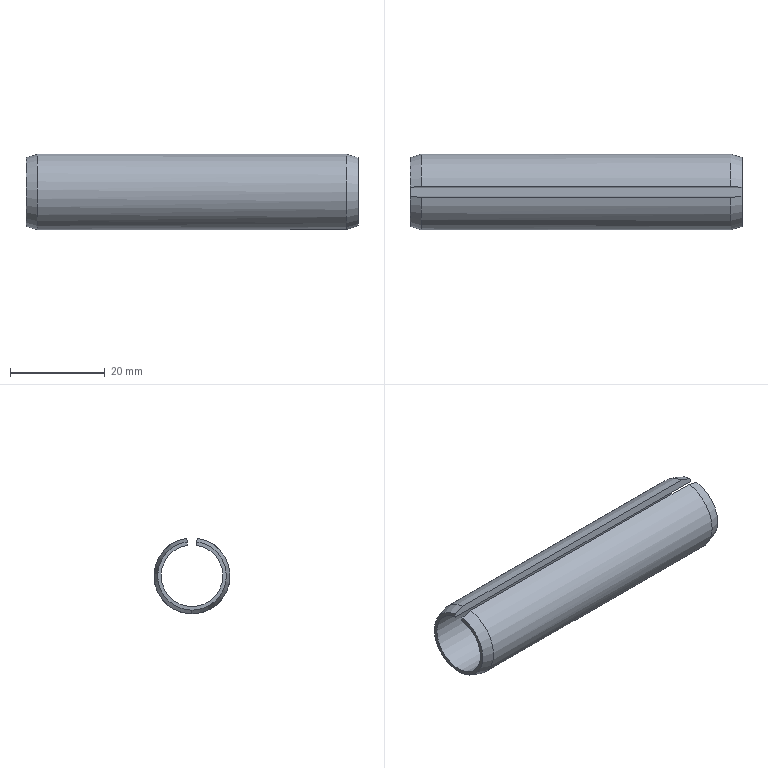Part | SolidWorks | features Boss 1, Cut 1, Extrusion 1, RevCut 1 | 1 solid | 9 faces | box 70 x 16 x 15.922 mm | volume 4487 mm3 | plane 4 | cone 3 | cylinder 2 | commonest cylinder face diameters 13 x1 16 x1
STEP:
#1=CARTESIAN_POINT('',(0.,-1.009,7.179));
#2=VERTEX_POINT('',#1);
#3=CARTESIAN_POINT('',(0.,0.,-7.25));
#4=VERTEX_POINT('',#3);
#5=CARTESIAN_POINT('',(0.,0.,0.));
#6=DIRECTION('',(1.,0.,0.));
#7=DIRECTION('',(0.,0.,-1.));
#8=AXIS2_PLACEMENT_3D('',#5,#6,#7);
#9=CIRCLE('',#8,7.25);
#10=EDGE_CURVE('',#2,#4,#9,.T.);
#11=ORIENTED_EDGE('',*,*,#10,.T.);
#12=CARTESIAN_POINT('',(2.4,0.,-8.));
#13=VERTEX_POINT('',#12);
#14=CARTESIAN_POINT('',(0.,0.,-7.25));
#15=DIRECTION('',(0.9545,0.,-0.2983));
#16=VECTOR('',#15,1000.);
#17=LINE('',#14,#16);
#18=EDGE_CURVE('',#4,#13,#17,.T.);
#19=ORIENTED_EDGE('',*,*,#18,.T.);
#20=CARTESIAN_POINT('',(2.4,-1.113,7.922));
#21=VERTEX_POINT('',#20);
#22=CARTESIAN_POINT('',(2.4,0.,0.));
#23=DIRECTION('',(1.,0.,0.));
#24=DIRECTION('',(0.,0.,-1.));
#25=AXIS2_PLACEMENT_3D('',#22,#23,#24);
#26=CIRCLE('',#25,8.);
#27=EDGE_CURVE('',#21,#13,#26,.T.);
#28=ORIENTED_EDGE('',*,*,#27,.F.);
#29=CARTESIAN_POINT('',(-23.2,0.,0.));
#30=DIRECTION('',(0.9545,-0.04151,0.2954));
#31=VECTOR('',#30,1000.);
#32=LINE('',#29,#31);
#33=EDGE_CURVE('',#2,#21,#32,.T.);
#34=ORIENTED_EDGE('',*,*,#33,.F.);
#35=EDGE_LOOP('',(#11,#19,#28,#34));
#36=FACE_OUTER_BOUND('',#35,.T.);
#37=CARTESIAN_POINT('',(0.,0.,0.));
#38=DIRECTION('',(1.,0.,0.));
#39=DIRECTION('',(0.,0.,-1.));
#40=AXIS2_PLACEMENT_3D('',#37,#38,#39);
#41=CONICAL_SURFACE('',#40,7.25,0.3029);
#42=ADVANCED_FACE('',(#36),#41,.T.);
#43=CARTESIAN_POINT('',(70.,-0.9046,6.437));
#44=VERTEX_POINT('',#43);
#45=CARTESIAN_POINT('',(70.,0.9046,6.437));
#46=VERTEX_POINT('',#45);
#47=CARTESIAN_POINT('',(70.,0.,0.));
#48=DIRECTION('',(1.,0.,0.));
#49=DIRECTION('',(0.,0.,-1.));
#50=AXIS2_PLACEMENT_3D('',#47,#48,#49);
#51=CIRCLE('',#50,6.5);
#52=EDGE_CURVE('',#44,#46,#51,.T.);
#53=ORIENTED_EDGE('',*,*,#52,.F.);
#54=CARTESIAN_POINT('',(70.,-1.009,7.179));
#55=VERTEX_POINT('',#54);
#56=CARTESIAN_POINT('',(70.,0.,0.));
#57=DIRECTION('',(0.,0.1392,-0.9903));
#58=VECTOR('',#57,1000.);
#59=LINE('',#56,#58);
#60=EDGE_CURVE('',#55,#44,#59,.T.);
#61=ORIENTED_EDGE('',*,*,#60,.F.);
#62=CARTESIAN_POINT('',(70.,1.009,7.179));
#63=VERTEX_POINT('',#62);
#64=CARTESIAN_POINT('',(70.,0.,0.));
#65=DIRECTION('',(1.,0.,0.));
#66=DIRECTION('',(0.,0.,-1.));
#67=AXIS2_PLACEMENT_3D('',#64,#65,#66);
#68=CIRCLE('',#67,7.25);
#69=EDGE_CURVE('',#55,#63,#68,.T.);
#70=ORIENTED_EDGE('',*,*,#69,.T.);
#71=CARTESIAN_POINT('',(70.,0.,0.));
#72=DIRECTION('',(0.,0.1392,0.9903));
#73=VECTOR('',#72,1000.);
#74=LINE('',#71,#73);
#75=EDGE_CURVE('',#46,#63,#74,.T.);
#76=ORIENTED_EDGE('',*,*,#75,.F.);
#77=EDGE_LOOP('',(#53,#61,#70,#76));
#78=FACE_OUTER_BOUND('',#77,.T.);
#79=CARTESIAN_POINT('',(70.,0.,0.));
#80=DIRECTION('',(1.,0.,0.));
#81=DIRECTION('',(0.,0.,-1.));
#82=AXIS2_PLACEMENT_3D('',#79,#80,#81);
#83=PLANE('',#82);
#84=ADVANCED_FACE('',(#78),#83,.T.);
#85=CARTESIAN_POINT('',(0.,-0.9046,6.437));
#86=VERTEX_POINT('',#85);
#87=CARTESIAN_POINT('',(0.,0.,0.));
#88=DIRECTION('',(0.,0.1392,-0.9903));
#89=VECTOR('',#88,1000.);
#90=LINE('',#87,#89);
#91=EDGE_CURVE('',#2,#86,#90,.T.);
#92=ORIENTED_EDGE('',*,*,#91,.T.);
#93=CARTESIAN_POINT('',(0.,0.9046,6.437));
#94=VERTEX_POINT('',#93);
#95=CARTESIAN_POINT('',(0.,0.,0.));
#96=DIRECTION('',(1.,0.,0.));
#97=DIRECTION('',(0.,0.,-1.));
#98=AXIS2_PLACEMENT_3D('',#95,#96,#97);
#99=CIRCLE('',#98,6.5);
#100=EDGE_CURVE('',#86,#94,#99,.T.);
#101=ORIENTED_EDGE('',*,*,#100,.T.);
#102=CARTESIAN_POINT('',(0.,1.009,7.179));
#103=VERTEX_POINT('',#102);
#104=CARTESIAN_POINT('',(0.,0.,0.));
#105=DIRECTION('',(0.,0.1392,0.9903));
#106=VECTOR('',#105,1000.);
#107=LINE('',#104,#106);
#108=EDGE_CURVE('',#94,#103,#107,.T.);
#109=ORIENTED_EDGE('',*,*,#108,.T.);
#110=CARTESIAN_POINT('',(0.,0.,0.));
#111=DIRECTION('',(1.,0.,0.));
#112=DIRECTION('',(0.,0.,-1.));
#113=AXIS2_PLACEMENT_3D('',#110,#111,#112);
#114=CIRCLE('',#113,7.25);
#115=EDGE_CURVE('',#4,#103,#114,.T.);
#116=ORIENTED_EDGE('',*,*,#115,.F.);
#117=ORIENTED_EDGE('',*,*,#10,.F.);
#118=EDGE_LOOP('',(#92,#101,#109,#116,#117));
#119=FACE_OUTER_BOUND('',#118,.T.);
#120=CARTESIAN_POINT('',(0.,0.,0.));
#121=DIRECTION('',(1.,0.,0.));
#122=DIRECTION('',(0.,0.,-1.));
#123=AXIS2_PLACEMENT_3D('',#120,#121,#122);
#124=PLANE('',#123);
#125=ADVANCED_FACE('',(#119),#124,.F.);
#126=CARTESIAN_POINT('',(67.6,-1.113,7.922));
#127=VERTEX_POINT('',#126);
#128=CARTESIAN_POINT('',(70.,-1.113,7.922));
#129=DIRECTION('',(1.,0.,0.));
#130=VECTOR('',#129,1000.);
#131=LINE('',#128,#130);
#132=EDGE_CURVE('',#21,#127,#131,.T.);
#133=ORIENTED_EDGE('',*,*,#132,.F.);
#134=ORIENTED_EDGE('',*,*,#27,.T.);
#135=CARTESIAN_POINT('',(2.4,1.113,7.922));
#136=VERTEX_POINT('',#135);
#137=CARTESIAN_POINT('',(2.4,0.,0.));
#138=DIRECTION('',(1.,0.,0.));
#139=DIRECTION('',(0.,0.,-1.));
#140=AXIS2_PLACEMENT_3D('',#137,#138,#139);
#141=CIRCLE('',#140,8.);
#142=EDGE_CURVE('',#13,#136,#141,.T.);
#143=ORIENTED_EDGE('',*,*,#142,.T.);
#144=CARTESIAN_POINT('',(67.6,1.113,7.922));
#145=VERTEX_POINT('',#144);
#146=CARTESIAN_POINT('',(70.,1.113,7.922));
#147=DIRECTION('',(-1.,0.,0.));
#148=VECTOR('',#147,1000.);
#149=LINE('',#146,#148);
#150=EDGE_CURVE('',#145,#136,#149,.T.);
#151=ORIENTED_EDGE('',*,*,#150,.F.);
#152=CARTESIAN_POINT('',(67.6,0.,0.));
#153=DIRECTION('',(1.,0.,0.));
#154=DIRECTION('',(0.,0.,-1.));
#155=AXIS2_PLACEMENT_3D('',#152,#153,#154);
#156=CIRCLE('',#155,8.);
#157=EDGE_CURVE('',#127,#145,#156,.T.);
#158=ORIENTED_EDGE('',*,*,#157,.F.);
#159=EDGE_LOOP('',(#133,#134,#143,#151,#158));
#160=FACE_OUTER_BOUND('',#159,.T.);
#161=CARTESIAN_POINT('',(70.,0.,0.));
#162=DIRECTION('',(-1.,0.,0.));
#163=DIRECTION('',(0.,0.,1.));
#164=AXIS2_PLACEMENT_3D('',#161,#162,#163);
#165=CYLINDRICAL_SURFACE('',#164,8.);
#166=ADVANCED_FACE('',(#160),#165,.T.);
#167=ORIENTED_EDGE('',*,*,#100,.F.);
#168=CARTESIAN_POINT('',(90.506,-0.9046,6.437));
#169=DIRECTION('',(1.,0.,0.));
#170=VECTOR('',#169,1000.);
#171=LINE('',#168,#170);
#172=EDGE_CURVE('',#86,#44,#171,.T.);
#173=ORIENTED_EDGE('',*,*,#172,.T.);
#174=ORIENTED_EDGE('',*,*,#52,.T.);
#175=CARTESIAN_POINT('',(90.506,0.9046,6.437));
#176=DIRECTION('',(-1.,0.,0.));
#177=VECTOR('',#176,1000.);
#178=LINE('',#175,#177);
#179=EDGE_CURVE('',#46,#94,#178,.T.);
#180=ORIENTED_EDGE('',*,*,#179,.T.);
#181=EDGE_LOOP('',(#167,#173,#174,#180));
#182=FACE_OUTER_BOUND('',#181,.T.);
#183=CARTESIAN_POINT('',(90.506,0.,0.));
#184=DIRECTION('',(-1.,0.,0.));
#185=DIRECTION('',(0.,0.,1.));
#186=AXIS2_PLACEMENT_3D('',#183,#184,#185);
#187=CYLINDRICAL_SURFACE('',#186,6.5);
#188=ADVANCED_FACE('',(#182),#187,.F.);
#189=CARTESIAN_POINT('',(93.2,0.,0.));
#190=DIRECTION('',(0.9545,0.04151,-0.2954));
#191=VECTOR('',#190,1000.);
#192=LINE('',#189,#191);
#193=EDGE_CURVE('',#127,#55,#192,.T.);
#194=ORIENTED_EDGE('',*,*,#193,.F.);
#195=ORIENTED_EDGE('',*,*,#157,.T.);
#196=CARTESIAN_POINT('',(93.2,0.,0.));
#197=DIRECTION('',(-0.9545,0.04151,0.2954));
#198=VECTOR('',#197,1000.);
#199=LINE('',#196,#198);
#200=EDGE_CURVE('',#63,#145,#199,.T.);
#201=ORIENTED_EDGE('',*,*,#200,.F.);
#202=ORIENTED_EDGE('',*,*,#69,.F.);
#203=EDGE_LOOP('',(#194,#195,#201,#202));
#204=FACE_OUTER_BOUND('',#203,.T.);
#205=CARTESIAN_POINT('',(67.6,0.,0.));
#206=DIRECTION('',(-1.,0.,0.));
#207=DIRECTION('',(0.,0.,1.));
#208=AXIS2_PLACEMENT_3D('',#205,#206,#207);
#209=CONICAL_SURFACE('',#208,8.,0.3029);
#210=ADVANCED_FACE('',(#204),#209,.T.);
#211=ORIENTED_EDGE('',*,*,#18,.F.);
#212=ORIENTED_EDGE('',*,*,#115,.T.);
#213=CARTESIAN_POINT('',(-23.2,0.,0.));
#214=DIRECTION('',(-0.9545,-0.04151,-0.2954));
#215=VECTOR('',#214,1000.);
#216=LINE('',#213,#215);
#217=EDGE_CURVE('',#136,#103,#216,.T.);
#218=ORIENTED_EDGE('',*,*,#217,.F.);
#219=ORIENTED_EDGE('',*,*,#142,.F.);
#220=EDGE_LOOP('',(#211,#212,#218,#219));
#221=FACE_OUTER_BOUND('',#220,.T.);
#222=CARTESIAN_POINT('',(0.,0.,0.));
#223=DIRECTION('',(1.,0.,0.));
#224=DIRECTION('',(0.,0.,-1.));
#225=AXIS2_PLACEMENT_3D('',#222,#223,#224);
#226=CONICAL_SURFACE('',#225,7.25,0.3029);
#227=ADVANCED_FACE('',(#221),#226,.T.);
#228=ORIENTED_EDGE('',*,*,#75,.T.);
#229=ORIENTED_EDGE('',*,*,#200,.T.);
#230=ORIENTED_EDGE('',*,*,#150,.T.);
#231=ORIENTED_EDGE('',*,*,#217,.T.);
#232=ORIENTED_EDGE('',*,*,#108,.F.);
#233=ORIENTED_EDGE('',*,*,#179,.F.);
#234=EDGE_LOOP('',(#228,#229,#230,#231,#232,#233));
#235=FACE_OUTER_BOUND('',#234,.T.);
#236=CARTESIAN_POINT('',(70.,0.,0.));
#237=DIRECTION('',(0.,-0.9903,0.1392));
#238=DIRECTION('',(0.,-0.1392,-0.9903));
#239=AXIS2_PLACEMENT_3D('',#236,#237,#238);
#240=PLANE('',#239);
#241=ADVANCED_FACE('',(#235),#240,.T.);
#242=ORIENTED_EDGE('',*,*,#91,.F.);
#243=ORIENTED_EDGE('',*,*,#33,.T.);
#244=ORIENTED_EDGE('',*,*,#132,.T.);
#245=ORIENTED_EDGE('',*,*,#193,.T.);
#246=ORIENTED_EDGE('',*,*,#60,.T.);
#247=ORIENTED_EDGE('',*,*,#172,.F.);
#248=EDGE_LOOP('',(#242,#243,#244,#245,#246,#247));
#249=FACE_OUTER_BOUND('',#248,.T.);
#250=CARTESIAN_POINT('',(70.,0.,0.));
#251=DIRECTION('',(0.,0.9903,0.1392));
#252=DIRECTION('',(0.,-0.1392,0.9903));
#253=AXIS2_PLACEMENT_3D('',#250,#251,#252);
#254=PLANE('',#253);
#255=ADVANCED_FACE('',(#249),#254,.T.);
#256=CLOSED_SHELL('',(#42,#84,#125,#166,#188,#210,#227,#241,#255));
#257=MANIFOLD_SOLID_BREP('',#256);
#258=CARTESIAN_POINT('',(0.,0.,0.));
#259=DIRECTION('',(0.,0.,1.));
#260=DIRECTION('',(1.,0.,0.));
#261=AXIS2_PLACEMENT_3D('',#258,#259,#260);
#262=(LENGTH_UNIT()NAMED_UNIT(*)SI_UNIT(.MILLI.,.METRE.));
#263=UNCERTAINTY_MEASURE_WITH_UNIT(LENGTH_MEASURE(0.00001),#262,'','');
#264=(NAMED_UNIT(*)PLANE_ANGLE_UNIT()SI_UNIT($,.RADIAN.));
#265=(NAMED_UNIT(*)SI_UNIT($,.STERADIAN.)SOLID_ANGLE_UNIT());
#266=(GEOMETRIC_REPRESENTATION_CONTEXT(3)GLOBAL_UNCERTAINTY_ASSIGNED_CONTEXT((#263))GLOBAL_UNIT_ASSIGNED_CONTEXT((#262,#264,#265))REPRESENTATION_CONTEXT('',''));
#267=ADVANCED_BREP_SHAPE_REPRESENTATION('',(#257,#261),#266);